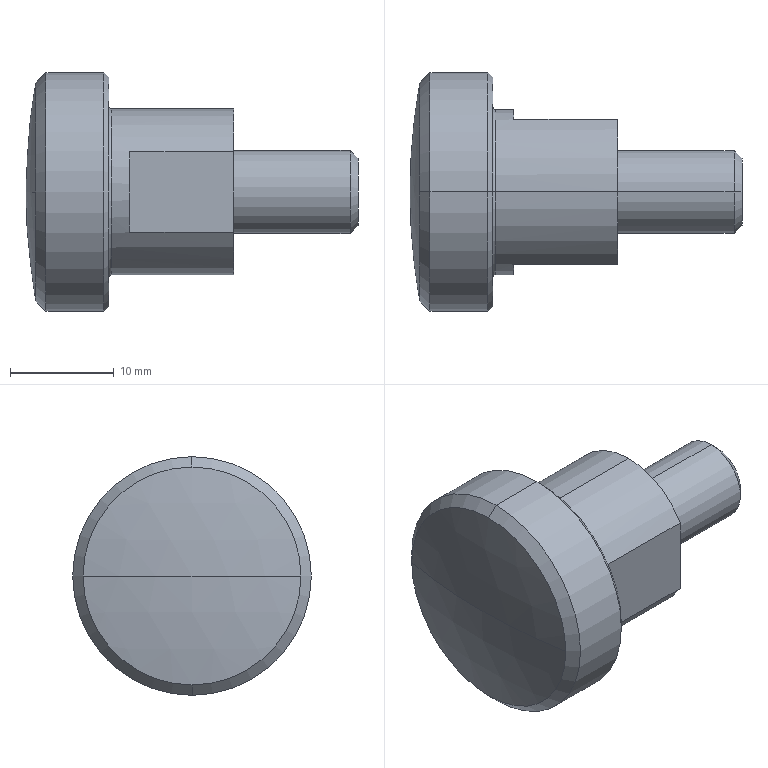Part | STEP file | qnSceondFJMC8part5 | 1 solid | 23 faces | box 32 x 23 x 23 mm | volume 5961 mm3 | plane 7 | cone 6 | cylinder 6 | torus 2 | sphere 2 | commonest cylinder face diameters 8 x2 16 x2 23 x2